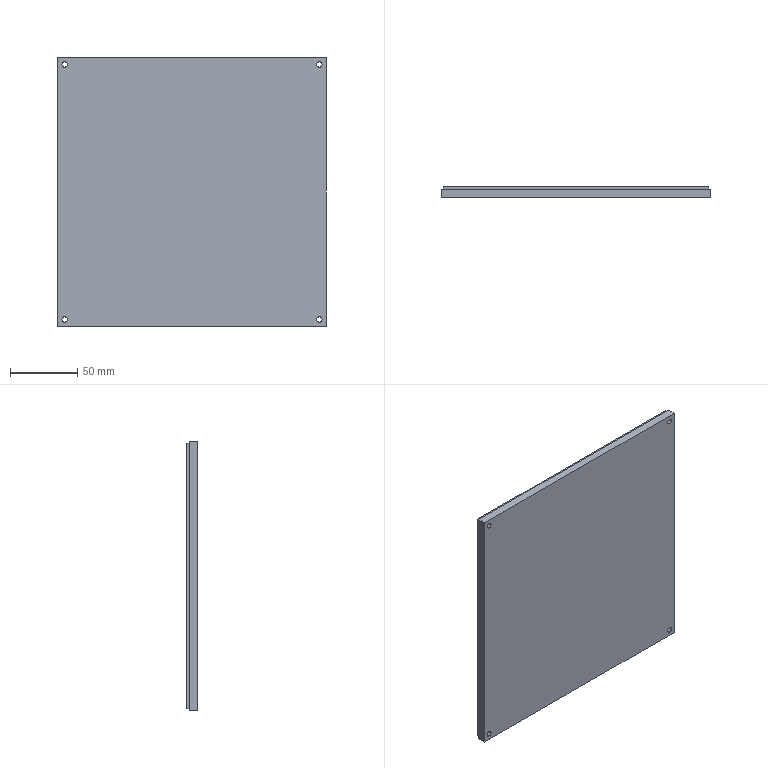Part | SolidWorks | features ICE 2, Extrusion 1, PLine 1 | 1 solid | 33 faces | box 200 x 8 x 200 mm | volume 318006 mm3 | plane 25 | cylinder 8 | commonest cylinder face diameters 4 x8